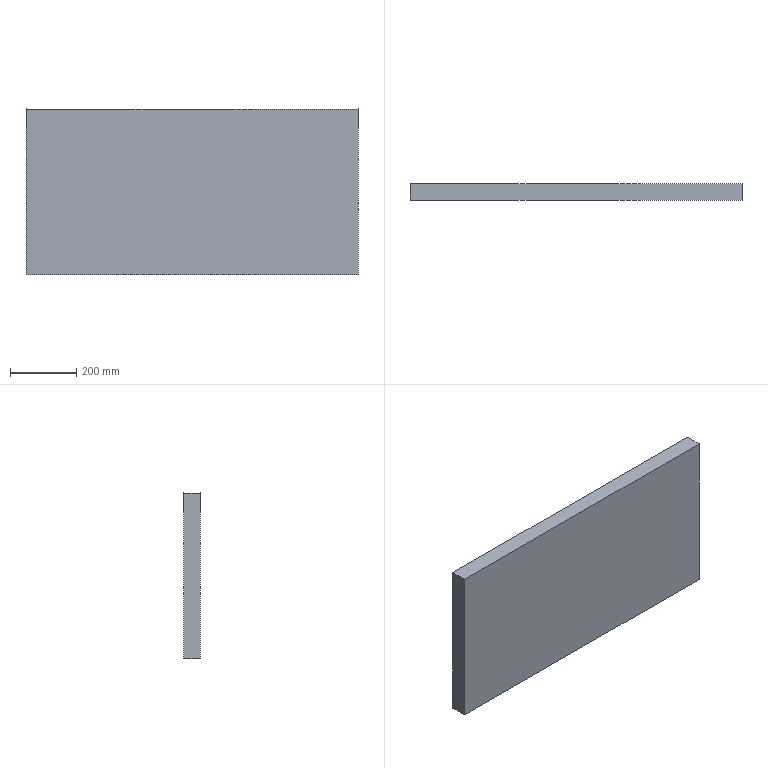Part | SolidWorks | features Extrusion 1 | 1 solid | 6 faces | box 1000 x 50 x 500 mm | volume 25000000 mm3 | plane 6
STEP:
#1=CARTESIAN_POINT('',(500.,0.,250.));
#2=VERTEX_POINT('',#1);
#3=CARTESIAN_POINT('',(500.,0.,-250.));
#4=VERTEX_POINT('',#3);
#5=CARTESIAN_POINT('',(500.,0.,-250.));
#6=DIRECTION('',(0.,0.,-1.));
#7=VECTOR('',#6,1000.);
#8=LINE('',#5,#7);
#9=EDGE_CURVE('',#2,#4,#8,.T.);
#10=ORIENTED_EDGE('',*,*,#9,.T.);
#11=CARTESIAN_POINT('',(500.,50.,-250.));
#12=VERTEX_POINT('',#11);
#13=CARTESIAN_POINT('',(500.,50.,-250.));
#14=DIRECTION('',(0.,-1.,0.));
#15=VECTOR('',#14,1000.);
#16=LINE('',#13,#15);
#17=EDGE_CURVE('',#12,#4,#16,.T.);
#18=ORIENTED_EDGE('',*,*,#17,.F.);
#19=CARTESIAN_POINT('',(500.,50.,250.));
#20=VERTEX_POINT('',#19);
#21=CARTESIAN_POINT('',(500.,50.,-250.));
#22=DIRECTION('',(0.,0.,-1.));
#23=VECTOR('',#22,1000.);
#24=LINE('',#21,#23);
#25=EDGE_CURVE('',#20,#12,#24,.T.);
#26=ORIENTED_EDGE('',*,*,#25,.F.);
#27=CARTESIAN_POINT('',(500.,50.,250.));
#28=DIRECTION('',(0.,-1.,0.));
#29=VECTOR('',#28,1000.);
#30=LINE('',#27,#29);
#31=EDGE_CURVE('',#20,#2,#30,.T.);
#32=ORIENTED_EDGE('',*,*,#31,.T.);
#33=EDGE_LOOP('',(#10,#18,#26,#32));
#34=FACE_OUTER_BOUND('',#33,.T.);
#35=CARTESIAN_POINT('',(500.,50.,-250.));
#36=DIRECTION('',(-1.,0.,0.));
#37=DIRECTION('',(0.,0.,1.));
#38=AXIS2_PLACEMENT_3D('',#35,#36,#37);
#39=PLANE('',#38);
#40=ADVANCED_FACE('',(#34),#39,.F.);
#41=CARTESIAN_POINT('',(-500.,0.,-250.));
#42=VERTEX_POINT('',#41);
#43=CARTESIAN_POINT('',(-500.,0.,-250.));
#44=DIRECTION('',(-1.,0.,0.));
#45=VECTOR('',#44,1000.);
#46=LINE('',#43,#45);
#47=EDGE_CURVE('',#4,#42,#46,.T.);
#48=ORIENTED_EDGE('',*,*,#47,.T.);
#49=CARTESIAN_POINT('',(-500.,50.,-250.));
#50=VERTEX_POINT('',#49);
#51=CARTESIAN_POINT('',(-500.,50.,-250.));
#52=DIRECTION('',(0.,-1.,0.));
#53=VECTOR('',#52,1000.);
#54=LINE('',#51,#53);
#55=EDGE_CURVE('',#50,#42,#54,.T.);
#56=ORIENTED_EDGE('',*,*,#55,.F.);
#57=CARTESIAN_POINT('',(-500.,50.,-250.));
#58=DIRECTION('',(-1.,0.,0.));
#59=VECTOR('',#58,1000.);
#60=LINE('',#57,#59);
#61=EDGE_CURVE('',#12,#50,#60,.T.);
#62=ORIENTED_EDGE('',*,*,#61,.F.);
#63=ORIENTED_EDGE('',*,*,#17,.T.);
#64=EDGE_LOOP('',(#48,#56,#62,#63));
#65=FACE_OUTER_BOUND('',#64,.T.);
#66=CARTESIAN_POINT('',(-500.,50.,-250.));
#67=DIRECTION('',(0.,0.,1.));
#68=DIRECTION('',(1.,0.,0.));
#69=AXIS2_PLACEMENT_3D('',#66,#67,#68);
#70=PLANE('',#69);
#71=ADVANCED_FACE('',(#65),#70,.F.);
#72=CARTESIAN_POINT('',(-500.,0.,250.));
#73=VERTEX_POINT('',#72);
#74=CARTESIAN_POINT('',(-500.,0.,-250.));
#75=DIRECTION('',(0.,0.,1.));
#76=VECTOR('',#75,1000.);
#77=LINE('',#74,#76);
#78=EDGE_CURVE('',#42,#73,#77,.T.);
#79=ORIENTED_EDGE('',*,*,#78,.T.);
#80=CARTESIAN_POINT('',(-500.,50.,250.));
#81=VERTEX_POINT('',#80);
#82=CARTESIAN_POINT('',(-500.,50.,250.));
#83=DIRECTION('',(0.,-1.,0.));
#84=VECTOR('',#83,1000.);
#85=LINE('',#82,#84);
#86=EDGE_CURVE('',#81,#73,#85,.T.);
#87=ORIENTED_EDGE('',*,*,#86,.F.);
#88=CARTESIAN_POINT('',(-500.,50.,-250.));
#89=DIRECTION('',(0.,0.,1.));
#90=VECTOR('',#89,1000.);
#91=LINE('',#88,#90);
#92=EDGE_CURVE('',#50,#81,#91,.T.);
#93=ORIENTED_EDGE('',*,*,#92,.F.);
#94=ORIENTED_EDGE('',*,*,#55,.T.);
#95=EDGE_LOOP('',(#79,#87,#93,#94));
#96=FACE_OUTER_BOUND('',#95,.T.);
#97=CARTESIAN_POINT('',(-500.,50.,-250.));
#98=DIRECTION('',(1.,0.,0.));
#99=DIRECTION('',(0.,0.,-1.));
#100=AXIS2_PLACEMENT_3D('',#97,#98,#99);
#101=PLANE('',#100);
#102=ADVANCED_FACE('',(#96),#101,.F.);
#103=CARTESIAN_POINT('',(-500.,0.,250.));
#104=DIRECTION('',(1.,0.,0.));
#105=VECTOR('',#104,1000.);
#106=LINE('',#103,#105);
#107=EDGE_CURVE('',#73,#2,#106,.T.);
#108=ORIENTED_EDGE('',*,*,#107,.T.);
#109=ORIENTED_EDGE('',*,*,#31,.F.);
#110=CARTESIAN_POINT('',(-500.,50.,250.));
#111=DIRECTION('',(1.,0.,0.));
#112=VECTOR('',#111,1000.);
#113=LINE('',#110,#112);
#114=EDGE_CURVE('',#81,#20,#113,.T.);
#115=ORIENTED_EDGE('',*,*,#114,.F.);
#116=ORIENTED_EDGE('',*,*,#86,.T.);
#117=EDGE_LOOP('',(#108,#109,#115,#116));
#118=FACE_OUTER_BOUND('',#117,.T.);
#119=CARTESIAN_POINT('',(-500.,50.,250.));
#120=DIRECTION('',(0.,0.,-1.));
#121=DIRECTION('',(-1.,0.,0.));
#122=AXIS2_PLACEMENT_3D('',#119,#120,#121);
#123=PLANE('',#122);
#124=ADVANCED_FACE('',(#118),#123,.F.);
#125=ORIENTED_EDGE('',*,*,#25,.T.);
#126=ORIENTED_EDGE('',*,*,#61,.T.);
#127=ORIENTED_EDGE('',*,*,#92,.T.);
#128=ORIENTED_EDGE('',*,*,#114,.T.);
#129=EDGE_LOOP('',(#125,#126,#127,#128));
#130=FACE_OUTER_BOUND('',#129,.T.);
#131=CARTESIAN_POINT('',(0.,50.,0.));
#132=DIRECTION('',(0.,1.,0.));
#133=DIRECTION('',(0.,0.,1.));
#134=AXIS2_PLACEMENT_3D('',#131,#132,#133);
#135=PLANE('',#134);
#136=ADVANCED_FACE('',(#130),#135,.T.);
#137=ORIENTED_EDGE('',*,*,#9,.F.);
#138=ORIENTED_EDGE('',*,*,#107,.F.);
#139=ORIENTED_EDGE('',*,*,#78,.F.);
#140=ORIENTED_EDGE('',*,*,#47,.F.);
#141=EDGE_LOOP('',(#137,#138,#139,#140));
#142=FACE_OUTER_BOUND('',#141,.T.);
#143=CARTESIAN_POINT('',(0.,0.,0.));
#144=DIRECTION('',(0.,1.,0.));
#145=DIRECTION('',(0.,0.,1.));
#146=AXIS2_PLACEMENT_3D('',#143,#144,#145);
#147=PLANE('',#146);
#148=ADVANCED_FACE('',(#142),#147,.F.);
#149=CLOSED_SHELL('',(#40,#71,#102,#124,#136,#148));
#150=MANIFOLD_SOLID_BREP('',#149);
#151=CARTESIAN_POINT('',(0.,0.,0.));
#152=DIRECTION('',(0.,0.,1.));
#153=DIRECTION('',(1.,0.,0.));
#154=AXIS2_PLACEMENT_3D('',#151,#152,#153);
#155=(LENGTH_UNIT()NAMED_UNIT(*)SI_UNIT(.MILLI.,.METRE.));
#156=UNCERTAINTY_MEASURE_WITH_UNIT(LENGTH_MEASURE(0.00001),#155,'','');
#157=(NAMED_UNIT(*)PLANE_ANGLE_UNIT()SI_UNIT($,.RADIAN.));
#158=(NAMED_UNIT(*)SI_UNIT($,.STERADIAN.)SOLID_ANGLE_UNIT());
#159=(GEOMETRIC_REPRESENTATION_CONTEXT(3)GLOBAL_UNCERTAINTY_ASSIGNED_CONTEXT((#156))GLOBAL_UNIT_ASSIGNED_CONTEXT((#155,#157,#158))REPRESENTATION_CONTEXT('',''));
#160=ADVANCED_BREP_SHAPE_REPRESENTATION('',(#150,#154),#159);